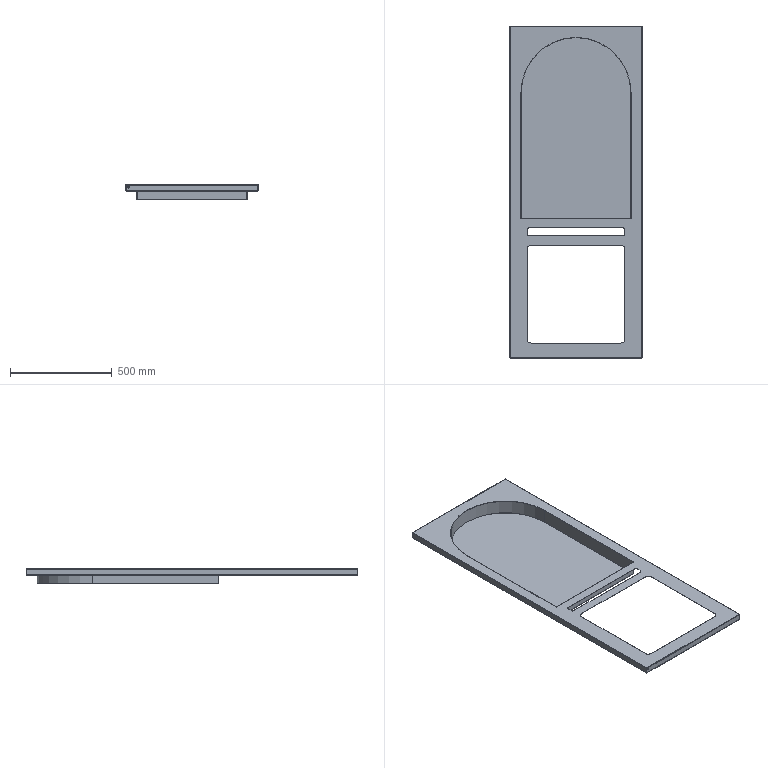Part | SolidWorks | features BaseBody 2 | 2 solids | 105 faces | box 648 x 1628 x 71.2 mm | volume 1419840 mm3 | plane 58 | cylinder 31 | spline 16 | commonest cylinder face diameters 2 x8 4.4 x8 8 x4 20 x4 40 x4 540 x2